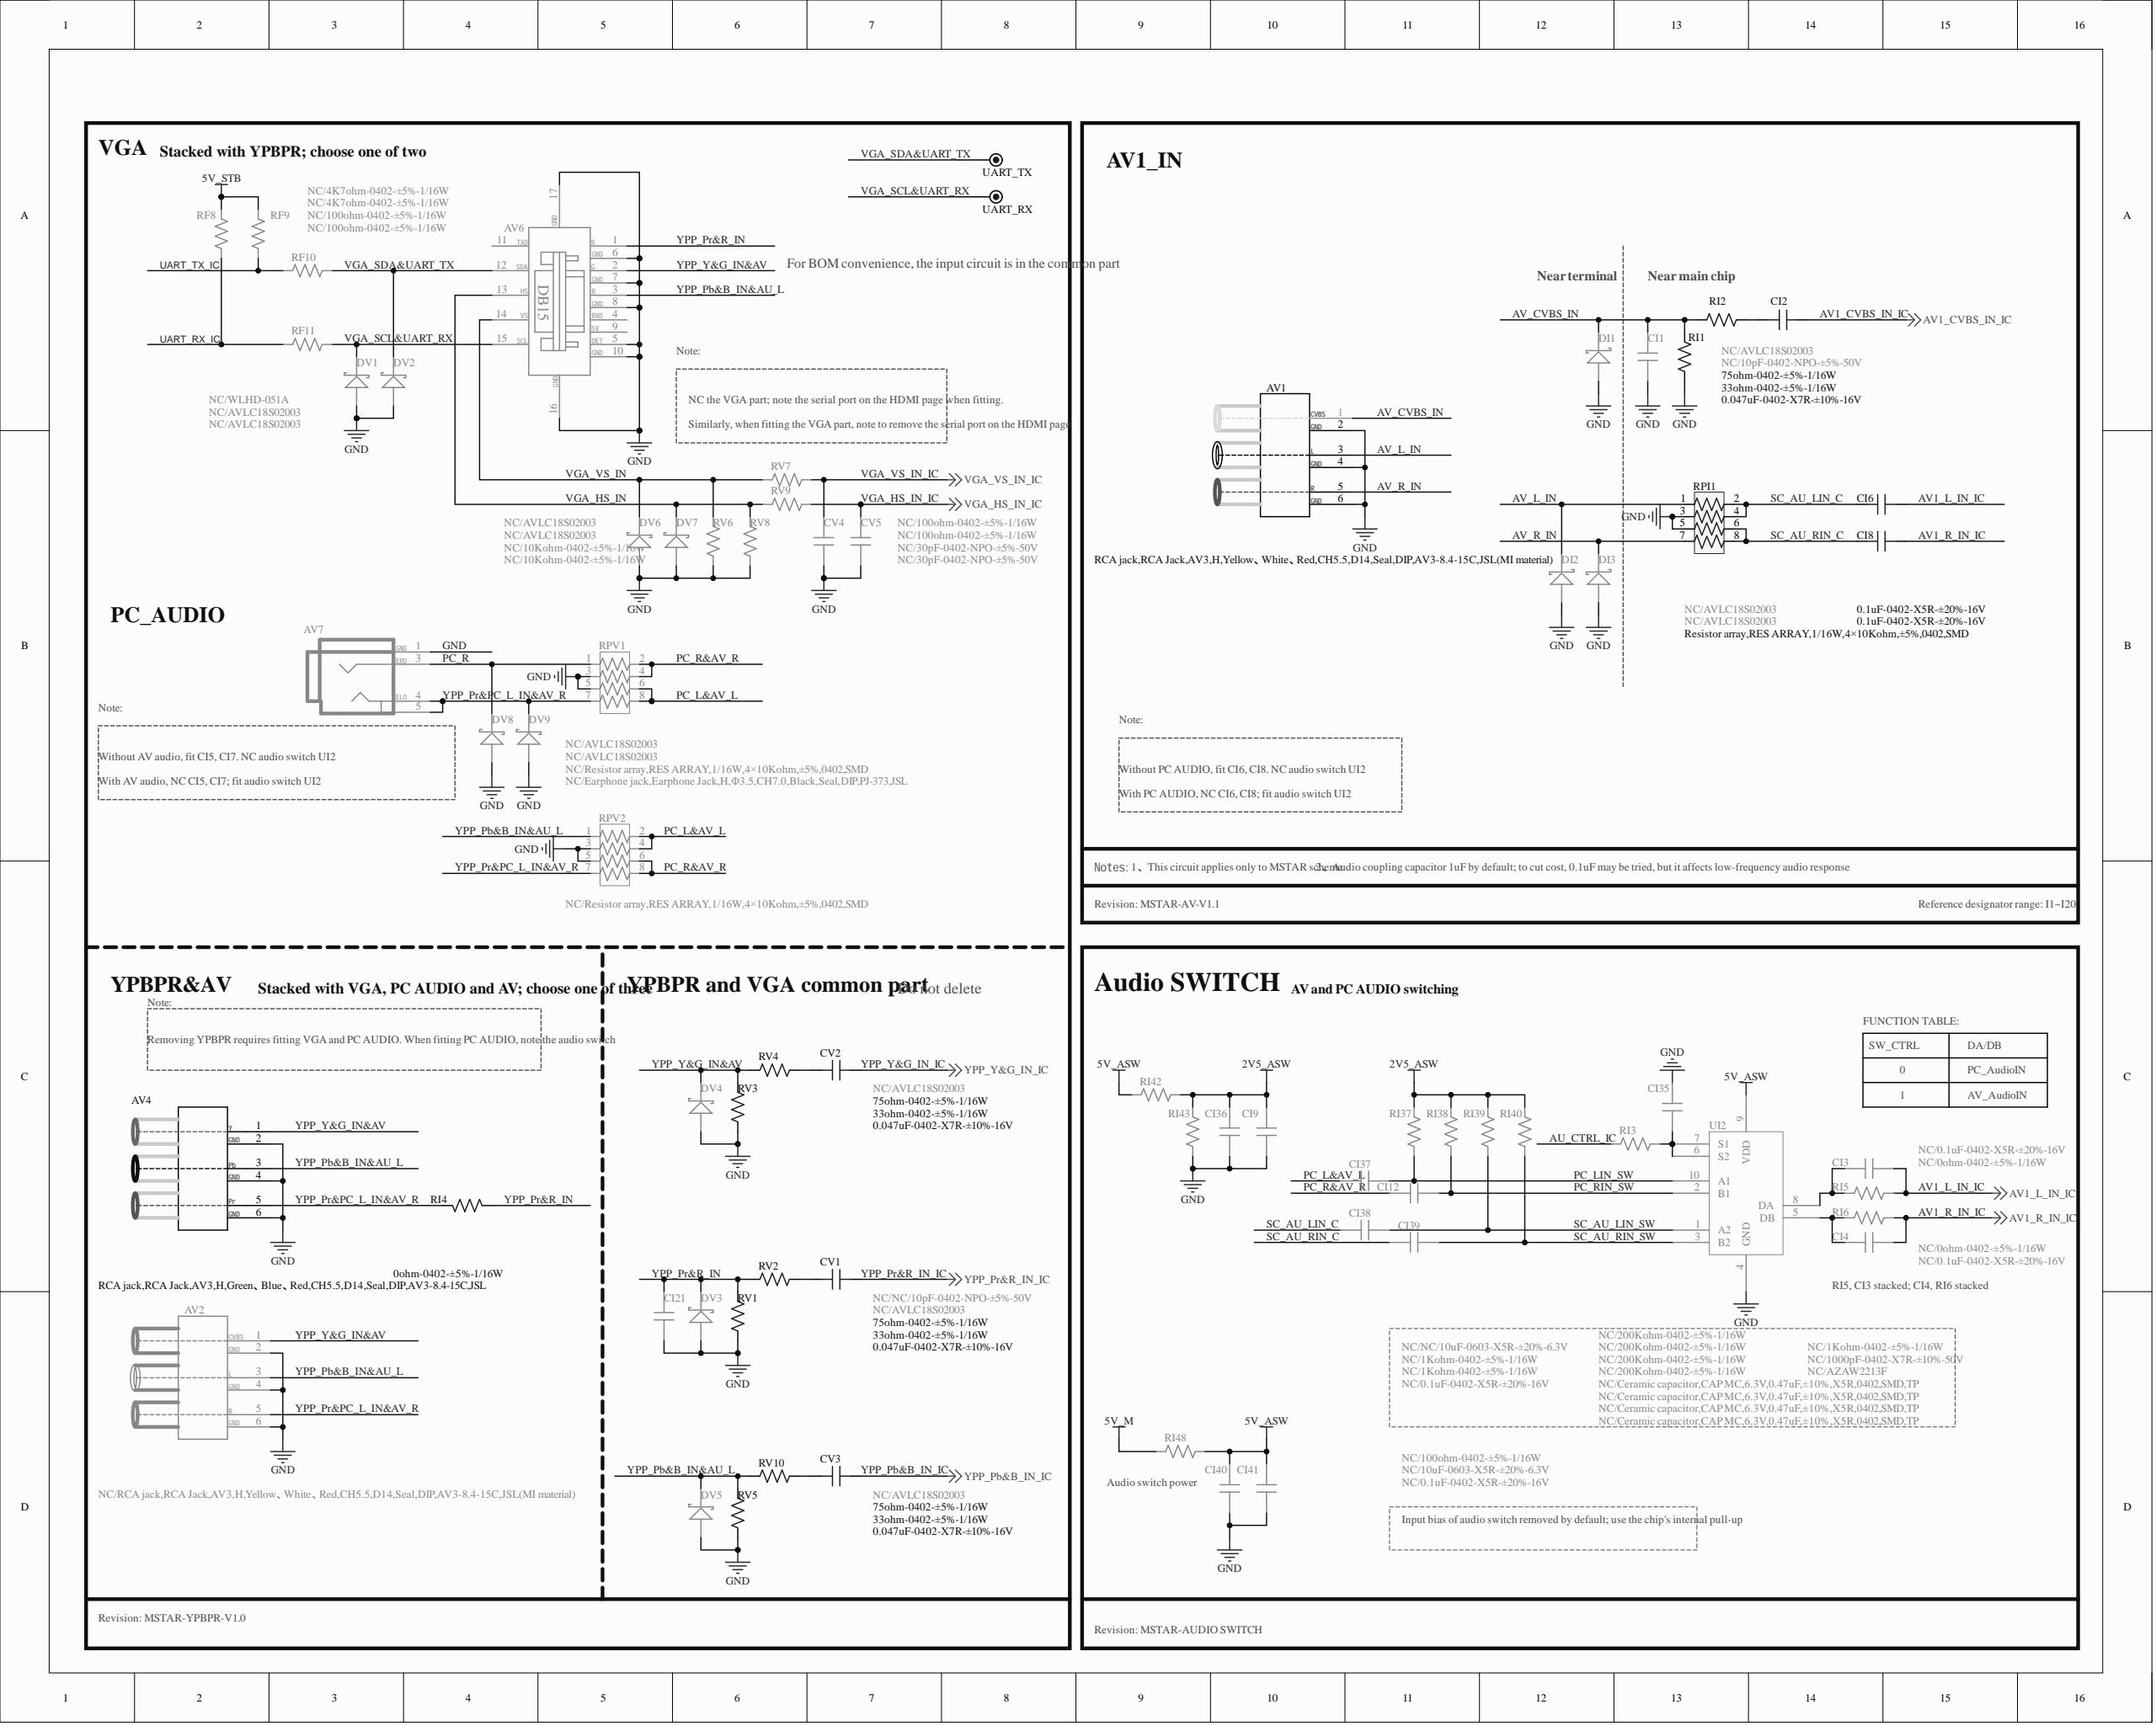Circuit board | Altium Designer | 578 parts | 300 nets | one sheet of the schematic
Parts on this sheet (reference | value | footprint):
AV1 | RCA jack,RCA Jack,AV3,H,Yellow、White、Red,CH5.5,D14,Seal,DIP,AV3-8.4-15C,JSL(MI material) | AV3-H14-15
AV2 | NC/RCA jack,RCA Jack,AV3,H,Yellow、White、Red,CH5.5,D14,Seal,DIP,AV3-8.4-15C,JSL(MI material) | AV3-H14-15
AV4 | RCA jack,RCA Jack,AV3,H,Green、Blue、Red,CH5.5,D14,Seal,DIP,AV3-8.4-15C,JSL | AV3-H14-15
AV6 | NC/WLHD-051A | DB15-HF-1
AV7 | NC/Earphone jack,Earphone Jack,H,F3.5,CH7.0,Black,Seal,DIP,PJ-373,JSL | PHONE-HD-41
CI1 | NC/10pF-0402-NPO-±5%-50V | C0402
CI2 | 0.047uF-0402-X7R-±10%-16V | C0402
CI3 | NC/0.1uF-0402-X5R-±20%-16V | C0402
CI4 | NC/0.1uF-0402-X5R-±20%-16V | C0402
CI6 | 0.1uF-0402-X5R-±20%-16V | C0402
CI8 | 0.1uF-0402-X5R-±20%-16V | C0402
CI9 | NC/NC/10uF-0603-X5R-±20%-6.3V | C0603
CI12 | NC/Ceramic capacitor,CAP MC,6.3V,0.47uF,±10%,X5R,0402,SMD,TP | C0402
CI21 | NC/NC/10pF-0402-NPO-±5%-50V | C0402
CI35 | NC/1000pF-0402-X7R-±10%-50V | C0402
CI36 | NC/0.1uF-0402-X5R-±20%-16V | C0402
CI37 | NC/Ceramic capacitor,CAP MC,6.3V,0.47uF,±10%,X5R,0402,SMD,TP | C0402
CI38 | NC/Ceramic capacitor,CAP MC,6.3V,0.47uF,±10%,X5R,0402,SMD,TP | C0402
CI39 | NC/Ceramic capacitor,CAP MC,6.3V,0.47uF,±10%,X5R,0402,SMD,TP | C0402
CI40 | NC/10uF-0603-X5R-±20%-6.3V | C0603
CI41 | NC/0.1uF-0402-X5R-±20%-16V | C0402
CV1 | 0.047uF-0402-X7R-±10%-16V | C0402
CV2 | 0.047uF-0402-X7R-±10%-16V | C0402
CV3 | 0.047uF-0402-X7R-±10%-16V | C0402
CV4 | NC/30pF-0402-NPO-±5%-50V | C0402
CV5 | NC/30pF-0402-NPO-±5%-50V | C0402
DI1 | NC/AVLC18S02003 | DIODE-S0402
DI2 | NC/AVLC18S02003 | DIODE-S0402
DI3 | NC/AVLC18S02003 | DIODE-S0402
DV1 | NC/AVLC18S02003 | DIODE-S0402
DV2 | NC/AVLC18S02003 | DIODE-S0402
DV3 | NC/AVLC18S02003 | DIODE-S0402
DV4 | NC/AVLC18S02003 | DIODE-S0402
DV5 | NC/AVLC18S02003 | DIODE-S0402
DV6 | NC/AVLC18S02003 | DIODE-S0402
DV7 | NC/AVLC18S02003 | DIODE-S0402
DV8 | NC/AVLC18S02003 | DIODE-S0402
DV9 | NC/AVLC18S02003 | DIODE-S0402
RF8 | NC/4K7ohm-0402-±5%-1/16W | R0402
RF9 | NC/4K7ohm-0402-±5%-1/16W | R0402
RF10 | NC/100ohm-0402-±5%-1/16W | R0402
RF11 | NC/100ohm-0402-±5%-1/16W | R0402
RI1 | 75ohm-0402-±5%-1/16W | R0402
RI2 | 33ohm-0402-±5%-1/16W | R0402
RI3 | NC/1Kohm-0402-±5%-1/16W | R0402
RI4 | 0ohm-0402-±5%-1/16W | R0402
RI5 | NC/0ohm-0402-±5%-1/16W | R0402
RI6 | NC/0ohm-0402-±5%-1/16W | R0402
RI37 | NC/200Kohm-0402-±5%-1/16W | R0402
RI38 | NC/200Kohm-0402-±5%-1/16W | R0402
RI39 | NC/200Kohm-0402-±5%-1/16W | R0402
RI40 | NC/200Kohm-0402-±5%-1/16W | R0402
RI42 | NC/1Kohm-0402-±5%-1/16W | R0402
RI43 | NC/1Kohm-0402-±5%-1/16W | R0402
RI48 | NC/100ohm-0402-±5%-1/16W | R0402
RPI1 | Resistor array,RES ARRAY,1/16W,4×10Kohm,±5%,0402,SMD | RA0402
RPV1 | NC/Resistor array,RES ARRAY,1/16W,4×10Kohm,±5%,0402,SMD | RA0402
RPV2 | NC/Resistor array,RES ARRAY,1/16W,4×10Kohm,±5%,0402,SMD | RA0402
RV1 | 75ohm-0402-±5%-1/16W | R0402
RV2 | 33ohm-0402-±5%-1/16W | R0402
RV3 | 75ohm-0402-±5%-1/16W | R0402
RV4 | 33ohm-0402-±5%-1/16W | R0402
RV5 | 75ohm-0402-±5%-1/16W | R0402
RV6 | NC/10Kohm-0402-±5%-1/16W | R0402
RV7 | NC/100ohm-0402-±5%-1/16W | R0402
RV8 | NC/10Kohm-0402-±5%-1/16W | R0402
RV9 | NC/100ohm-0402-±5%-1/16W | R0402
RV10 | 33ohm-0402-±5%-1/16W | R0402
UART_RX | DM0 | TP
UART_TX | DM0 | TP
UI2 | NC/AZAW2213F | QFN10/0.4
Nets of these parts (net: part-pin ...):
YPP_Y&G_IN_IC: CV2-2
YPP_Y&G_IN&AV: AV2-1 AV4-1 AV6-2 DV4-K RV3-2 RV4-1
YPP_Pr&R_IN_IC: CV1-2
YPP_Pr&R_IN: AV6-1 CI21-1 DV3-K RI4-1 RV1-2 RV2-1
YPP_Pr&PC_L_IN&AV_R: AV2-5 AV4-5 AV7-4 AV7-5 DV9-K RI4-2 RPV1-7 RPV2-7
YPP_Pb&B_IN_IC: CV3-2
YPP_Pb&B_IN&AU_L: AV2-3 AV4-3 AV6-3 DV5-K RPV2-1 RV5-2 RV10-1
VGA_VS_IN_IC: CV4-2 RV7-2
VGA_VS_IN: AV6-14 DV6-K RV6-2 RV7-1
VGA_SDA&UART_TX: AV6-12 DV2-K RF10-2 UART_TX-1
VGA_SCL&UART_RX: AV6-15 DV1-K RF11-2 UART_RX-1
VGA_HS_IN_IC: CV5-2 RV9-2
VGA_HS_IN: AV6-13 DV7-K RV8-2 RV9-1
UART_TX_IC: RF9-1 RF10-1
UART_RX_IC: RF8-1 RF11-1
SC_AU_RIN_SW: CI39-1 RI40-1 UI2-3
SC_AU_RIN_C: CI8-2 CI39-2 RPI1-6 RPI1-8
SC_AU_LIN_SW: CI38-1 RI39-1 UI2-1
SC_AU_LIN_C: CI6-2 CI38-2 RPI1-2 RPI1-4
PC_RIN_SW: CI12-1 RI38-1 UI2-2
PC_R&AV_R: CI12-2 RPV1-2 RPV1-4 RPV2-6 RPV2-8
PC_R: AV7-3 DV8-K RPV1-1
PC_LIN_SW: CI37-1 RI37-1 UI2-10
PC_L&AV_L: CI37-2 RPV1-6 RPV1-8 RPV2-2 RPV2-4
NetCV3_1: CV3-1 RV10-2
NetCV2_1: CV2-1 RV4-2
NetCV1_1: CV1-1 RV2-2
NetCI35_1: CI35-1 RI3-2 UI2-6 UI2-7
NetCI4_2: CI4-2 RI6-1 UI2-5
NetCI3_2: CI3-2 RI5-1 UI2-8
NetCI2_1: CI2-1 RI2-1
GND: AV1-2 AV1-4 AV1-6 AV2-2 AV2-4 AV2-6 AV4-2 AV4-4 AV4-6 AV6-5 AV6-6 AV6-7 AV6-8 AV6-10 AV6-16 AV6-17 AV7-1 CI1-2 CI9-1 CI21-2 CI35-2 CI36-1 CI40-1 CI41-1 CV4-1 CV5-1 DI1-A DI2-A DI3-A DV1-A DV2-A DV3-A DV4-A DV5-A DV6-A DV7-A DV8-A DV9-A RI1-1 RI43-1 RPI1-3 RPI1-5 RPV1-3 RPV1-5 RPV2-3 RPV2-5 RV1-1 RV3-1 RV5-1 RV6-1 RV8-1 UI2-4
AV_R_IN: AV1-5 DI3-K RPI1-7
AV_L_IN: AV1-3 DI2-K RPI1-1
AV_CVBS_IN: AV1-1 CI1-1 DI1-K RI1-2 RI2-2
AV1_R_IN_IC: CI4-1 CI8-1 RI6-2
AV1_L_IN_IC: CI3-1 CI6-1 RI5-2
AV1_CVBS_IN_IC: CI2-2
AU_CTRL_IC: RI3-1
5V_STB: RF8-2 RF9-2
5V_M: RI48-1
5V_ASW: CI40-2 CI41-2 RI42-1 RI48-2 UI2-9
2V5_ASW: CI9-2 CI36-2 RI37-2 RI38-2 RI39-2 RI40-2 RI42-2 RI43-2